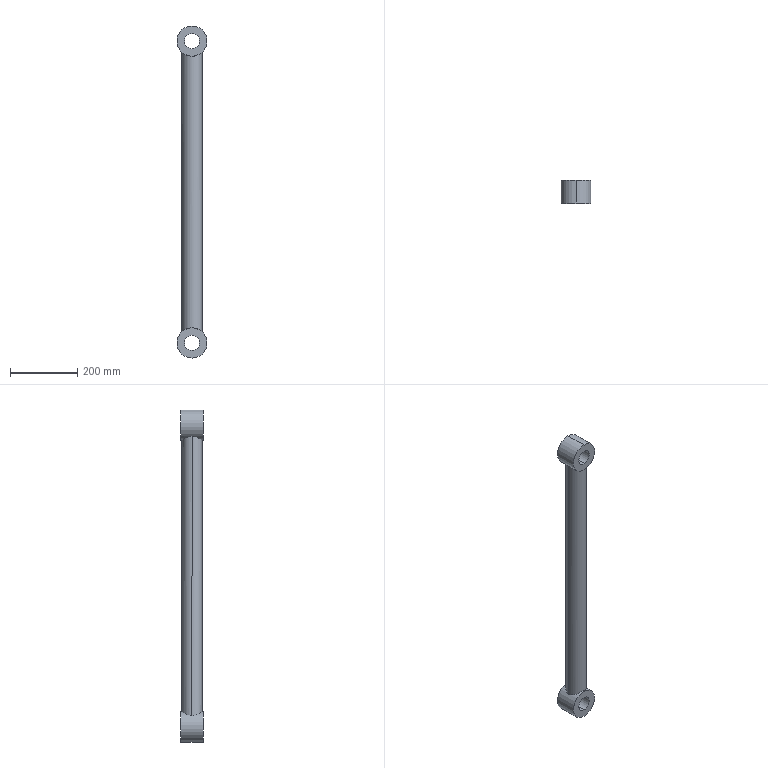Part | SolidWorks | features ICE 2, Extrusion 1, Scale 1 | 1 solid | 14 faces | box 90 x 67.5 x 990 mm | volume 2949409 mm3 | cylinder 10 | plane 4 | commonest cylinder face diameters 45 x4 90 x4 60 x2
STEP:
#1=CARTESIAN_POINT('',(0.00000416,33.75,-472.5));
#2=VERTEX_POINT('',#1);
#3=CARTESIAN_POINT('',(0.00000416,33.75,-427.5));
#4=VERTEX_POINT('',#3);
#5=CARTESIAN_POINT('',(0.00000416,33.75,-450.));
#6=DIRECTION('',(0.,1.,0.));
#7=DIRECTION('',(0.,0.,-1.));
#8=AXIS2_PLACEMENT_3D('',#5,#6,#7);
#9=CIRCLE('',#8,22.5);
#10=EDGE_CURVE('',#2,#4,#9,.T.);
#11=ORIENTED_EDGE('',*,*,#10,.T.);
#12=CARTESIAN_POINT('',(0.00000416,-33.75,-427.5));
#13=VERTEX_POINT('',#12);
#14=CARTESIAN_POINT('',(0.00000416,33.75,-427.5));
#15=DIRECTION('',(0.,-1.,0.));
#16=VECTOR('',#15,1000.);
#17=LINE('',#14,#16);
#18=EDGE_CURVE('',#4,#13,#17,.T.);
#19=ORIENTED_EDGE('',*,*,#18,.T.);
#20=CARTESIAN_POINT('',(0.00000416,-33.75,-472.5));
#21=VERTEX_POINT('',#20);
#22=CARTESIAN_POINT('',(0.00000416,-33.75,-450.));
#23=DIRECTION('',(0.,1.,0.));
#24=DIRECTION('',(0.,0.,-1.));
#25=AXIS2_PLACEMENT_3D('',#22,#23,#24);
#26=CIRCLE('',#25,22.5);
#27=EDGE_CURVE('',#21,#13,#26,.T.);
#28=ORIENTED_EDGE('',*,*,#27,.F.);
#29=CARTESIAN_POINT('',(0.00000416,33.75,-472.5));
#30=DIRECTION('',(0.,-1.,0.));
#31=VECTOR('',#30,1000.);
#32=LINE('',#29,#31);
#33=EDGE_CURVE('',#2,#21,#32,.T.);
#34=ORIENTED_EDGE('',*,*,#33,.F.);
#35=EDGE_LOOP('',(#11,#19,#28,#34));
#36=FACE_OUTER_BOUND('',#35,.T.);
#37=CARTESIAN_POINT('',(0.00000416,33.75,-450.));
#38=DIRECTION('',(0.,-1.,0.));
#39=DIRECTION('',(0.,0.,-1.));
#40=AXIS2_PLACEMENT_3D('',#37,#38,#39);
#41=CYLINDRICAL_SURFACE('',#40,22.5);
#42=ADVANCED_FACE('',(#36),#41,.F.);
#43=CARTESIAN_POINT('',(0.00000416,33.75,-405.));
#44=VERTEX_POINT('',#43);
#45=CARTESIAN_POINT('',(0.00000416,33.75,-495.));
#46=VERTEX_POINT('',#45);
#47=CARTESIAN_POINT('',(0.00000416,33.75,-450.));
#48=DIRECTION('',(0.,1.,0.));
#49=DIRECTION('',(0.,0.,-1.));
#50=AXIS2_PLACEMENT_3D('',#47,#48,#49);
#51=CIRCLE('',#50,45.);
#52=EDGE_CURVE('',#44,#46,#51,.T.);
#53=ORIENTED_EDGE('',*,*,#52,.F.);
#54=CARTESIAN_POINT('',(0.00000416,30.,-405.));
#55=VERTEX_POINT('',#54);
#56=CARTESIAN_POINT('',(0.00000416,33.75,-405.));
#57=DIRECTION('',(0.,-1.,0.));
#58=VECTOR('',#57,1000.);
#59=LINE('',#56,#58);
#60=EDGE_CURVE('',#44,#55,#59,.T.);
#61=ORIENTED_EDGE('',*,*,#60,.T.);
#62=CARTESIAN_POINT('',(30.,0.00002262,-416.459));
#63=VERTEX_POINT('',#62);
#64=CARTESIAN_POINT('',(0.00000416,30.,-405.));
#65=CARTESIAN_POINT('',(0.5109,30.,-405.));
#66=CARTESIAN_POINT('',(1.025,29.987,-405.009));
#67=CARTESIAN_POINT('',(2.044,29.935,-405.043));
#68=CARTESIAN_POINT('',(2.55,29.896,-405.069));
#69=CARTESIAN_POINT('',(4.059,29.741,-405.172));
#70=CARTESIAN_POINT('',(5.054,29.588,-405.274));
#71=CARTESIAN_POINT('',(7.02,29.184,-405.54));
#72=CARTESIAN_POINT('',(7.992,28.933,-405.704));
#73=CARTESIAN_POINT('',(9.913,28.333,-406.094));
#74=CARTESIAN_POINT('',(10.847,27.988,-406.317));
#75=CARTESIAN_POINT('',(12.659,27.216,-406.807));
#76=CARTESIAN_POINT('',(13.538,26.789,-407.075));
#77=CARTESIAN_POINT('',(14.82,26.089,-407.508));
#78=CARTESIAN_POINT('',(15.241,25.845,-407.657));
#79=CARTESIAN_POINT('',(16.07,25.338,-407.965));
#80=CARTESIAN_POINT('',(16.479,25.073,-408.124));
#81=CARTESIAN_POINT('',(18.483,23.709,-408.935));
#82=CARTESIAN_POINT('',(19.945,22.49,-409.633));
#83=CARTESIAN_POINT('',(21.951,20.471,-410.71));
#84=CARTESIAN_POINT('',(22.589,19.765,-411.074));
#85=CARTESIAN_POINT('',(23.801,18.288,-411.803));
#86=CARTESIAN_POINT('',(24.369,17.523,-412.164));
#87=CARTESIAN_POINT('',(25.958,15.158,-413.22));
#88=CARTESIAN_POINT('',(26.868,13.486,-413.888));
#89=CARTESIAN_POINT('',(27.814,11.252,-414.624));
#90=CARTESIAN_POINT('',(27.994,10.798,-414.766));
#91=CARTESIAN_POINT('',(28.333,9.875,-415.038));
#92=CARTESIAN_POINT('',(28.492,9.403,-415.169));
#93=CARTESIAN_POINT('',(28.936,7.981,-415.534));
#94=CARTESIAN_POINT('',(29.184,7.019,-415.746));
#95=CARTESIAN_POINT('',(29.587,5.063,-416.093));
#96=CARTESIAN_POINT('',(29.74,4.069,-416.228));
#97=CARTESIAN_POINT('',(29.895,2.553,-416.366));
#98=CARTESIAN_POINT('',(29.935,2.042,-416.401));
#99=CARTESIAN_POINT('',(29.987,1.019,-416.447));
#100=CARTESIAN_POINT('',(30.,0.5084,-416.459));
#101=CARTESIAN_POINT('',(30.,0.00002262,-416.459));
#102=B_SPLINE_CURVE_WITH_KNOTS('',3,(#64,#65,#66,#67,#68,#69,#70,#71,#72,#73,#74,#75,#76,#77,#78,#79,#80,#81,#82,#83,#84,#85,#86,#87,#88,#89,#90,#91,#92,#93,#94,#95,#96,#97,#98,#99,#100,#101),.UNSPECIFIED.,.F.,.F.,(4,2,2,2,2,2,2,2,2,2,2,2,2,2,2,2,2,2,4),(0.04853,0.05004,0.05155,0.05457,0.05759,0.06062,0.06364,0.06515,0.06666,0.07271,0.07573,0.07876,0.0848,0.08631,0.08783,0.09085,0.09387,0.09538,0.0969),.UNSPECIFIED.);
#103=EDGE_CURVE('',#55,#63,#102,.T.);
#104=ORIENTED_EDGE('',*,*,#103,.T.);
#105=CARTESIAN_POINT('',(0.00000416,-30.,-405.));
#106=VERTEX_POINT('',#105);
#107=CARTESIAN_POINT('',(30.,0.00002262,-416.459));
#108=CARTESIAN_POINT('',(30.,-2.032,-416.459));
#109=CARTESIAN_POINT('',(29.796,-4.037,-416.273));
#110=CARTESIAN_POINT('',(29.289,-6.511,-415.836));
#111=CARTESIAN_POINT('',(29.176,-7.001,-415.739));
#112=CARTESIAN_POINT('',(28.927,-7.968,-415.529));
#113=CARTESIAN_POINT('',(28.791,-8.445,-415.415));
#114=CARTESIAN_POINT('',(28.351,-9.859,-415.052));
#115=CARTESIAN_POINT('',(28.014,-10.778,-414.78));
#116=CARTESIAN_POINT('',(27.255,-12.574,-414.189));
#117=CARTESIAN_POINT('',(26.831,-13.455,-413.869));
#118=CARTESIAN_POINT('',(25.911,-15.15,-413.204));
#119=CARTESIAN_POINT('',(25.416,-15.967,-412.859));
#120=CARTESIAN_POINT('',(24.353,-17.546,-412.153));
#121=CARTESIAN_POINT('',(23.785,-18.307,-411.793));
#122=CARTESIAN_POINT('',(22.578,-19.778,-411.067));
#123=CARTESIAN_POINT('',(21.934,-20.489,-410.7));
#124=CARTESIAN_POINT('',(19.917,-22.516,-409.619));
#125=CARTESIAN_POINT('',(18.457,-23.728,-408.923));
#126=CARTESIAN_POINT('',(16.079,-25.345,-407.962));
#127=CARTESIAN_POINT('',(15.255,-25.851,-407.655));
#128=CARTESIAN_POINT('',(13.967,-26.555,-407.22));
#129=CARTESIAN_POINT('',(13.528,-26.781,-407.079));
#130=CARTESIAN_POINT('',(12.64,-27.212,-406.809));
#131=CARTESIAN_POINT('',(12.191,-27.416,-406.68));
#132=CARTESIAN_POINT('',(9.921,-28.381,-406.067));
#133=CARTESIAN_POINT('',(8.025,-28.977,-405.676));
#134=CARTESIAN_POINT('',(5.545,-29.487,-405.34));
#135=CARTESIAN_POINT('',(5.042,-29.578,-405.28));
#136=CARTESIAN_POINT('',(4.035,-29.732,-405.178));
#137=CARTESIAN_POINT('',(3.532,-29.796,-405.136));
#138=CARTESIAN_POINT('',(2.02,-29.949,-405.034));
#139=CARTESIAN_POINT('',(1.011,-30.,-405.));
#140=CARTESIAN_POINT('',(0.00000416,-30.,-405.));
#141=B_SPLINE_CURVE_WITH_KNOTS('',3,(#107,#108,#109,#110,#111,#112,#113,#114,#115,#116,#117,#118,#119,#120,#121,#122,#123,#124,#125,#126,#127,#128,#129,#130,#131,#132,#133,#134,#135,#136,#137,#138,#139,#140),.UNSPECIFIED.,.F.,.F.,(4,2,2,2,2,2,2,2,2,2,2,2,2,2,2,2,4),(0.0969,0.1029,0.1044,0.106,0.109,0.112,0.115,0.118,0.1211,0.1271,0.1301,0.1316,0.1331,0.1392,0.1407,0.1422,0.1452),.UNSPECIFIED.);
#142=EDGE_CURVE('',#63,#106,#141,.T.);
#143=ORIENTED_EDGE('',*,*,#142,.T.);
#144=CARTESIAN_POINT('',(0.00000416,-33.75,-405.));
#145=VERTEX_POINT('',#144);
#146=CARTESIAN_POINT('',(0.00000416,33.75,-405.));
#147=DIRECTION('',(0.,-1.,0.));
#148=VECTOR('',#147,1000.);
#149=LINE('',#146,#148);
#150=EDGE_CURVE('',#106,#145,#149,.T.);
#151=ORIENTED_EDGE('',*,*,#150,.T.);
#152=CARTESIAN_POINT('',(0.00000416,-33.75,-495.));
#153=VERTEX_POINT('',#152);
#154=CARTESIAN_POINT('',(0.00000416,-33.75,-450.));
#155=DIRECTION('',(0.,1.,0.));
#156=DIRECTION('',(0.,0.,-1.));
#157=AXIS2_PLACEMENT_3D('',#154,#155,#156);
#158=CIRCLE('',#157,45.);
#159=EDGE_CURVE('',#145,#153,#158,.T.);
#160=ORIENTED_EDGE('',*,*,#159,.T.);
#161=CARTESIAN_POINT('',(0.00000416,33.75,-495.));
#162=DIRECTION('',(0.,-1.,0.));
#163=VECTOR('',#162,1000.);
#164=LINE('',#161,#163);
#165=EDGE_CURVE('',#46,#153,#164,.T.);
#166=ORIENTED_EDGE('',*,*,#165,.F.);
#167=EDGE_LOOP('',(#53,#61,#104,#143,#151,#160,#166));
#168=FACE_OUTER_BOUND('',#167,.T.);
#169=CARTESIAN_POINT('',(0.00000416,33.75,-450.));
#170=DIRECTION('',(0.,-1.,0.));
#171=DIRECTION('',(0.,0.,-1.));
#172=AXIS2_PLACEMENT_3D('',#169,#170,#171);
#173=CYLINDRICAL_SURFACE('',#172,45.);
#174=ADVANCED_FACE('',(#168),#173,.T.);
#175=CARTESIAN_POINT('',(0.00000416,33.75,427.5));
#176=VERTEX_POINT('',#175);
#177=CARTESIAN_POINT('',(0.00000416,33.75,472.5));
#178=VERTEX_POINT('',#177);
#179=CARTESIAN_POINT('',(0.00000416,33.75,450.));
#180=DIRECTION('',(0.,1.,0.));
#181=DIRECTION('',(0.,0.,1.));
#182=AXIS2_PLACEMENT_3D('',#179,#180,#181);
#183=CIRCLE('',#182,22.5);
#184=EDGE_CURVE('',#176,#178,#183,.T.);
#185=ORIENTED_EDGE('',*,*,#184,.T.);
#186=CARTESIAN_POINT('',(0.00000416,-33.75,472.5));
#187=VERTEX_POINT('',#186);
#188=CARTESIAN_POINT('',(0.00000416,33.75,472.5));
#189=DIRECTION('',(0.,-1.,0.));
#190=VECTOR('',#189,1000.);
#191=LINE('',#188,#190);
#192=EDGE_CURVE('',#178,#187,#191,.T.);
#193=ORIENTED_EDGE('',*,*,#192,.T.);
#194=CARTESIAN_POINT('',(0.00000416,-33.75,427.5));
#195=VERTEX_POINT('',#194);
#196=CARTESIAN_POINT('',(0.00000416,-33.75,450.));
#197=DIRECTION('',(0.,1.,0.));
#198=DIRECTION('',(0.,0.,1.));
#199=AXIS2_PLACEMENT_3D('',#196,#197,#198);
#200=CIRCLE('',#199,22.5);
#201=EDGE_CURVE('',#195,#187,#200,.T.);
#202=ORIENTED_EDGE('',*,*,#201,.F.);
#203=CARTESIAN_POINT('',(0.00000416,33.75,427.5));
#204=DIRECTION('',(0.,-1.,0.));
#205=VECTOR('',#204,1000.);
#206=LINE('',#203,#205);
#207=EDGE_CURVE('',#176,#195,#206,.T.);
#208=ORIENTED_EDGE('',*,*,#207,.F.);
#209=EDGE_LOOP('',(#185,#193,#202,#208));
#210=FACE_OUTER_BOUND('',#209,.T.);
#211=CARTESIAN_POINT('',(0.00000416,33.75,450.));
#212=DIRECTION('',(0.,-1.,0.));
#213=DIRECTION('',(0.,0.,-1.));
#214=AXIS2_PLACEMENT_3D('',#211,#212,#213);
#215=CYLINDRICAL_SURFACE('',#214,22.5);
#216=ADVANCED_FACE('',(#210),#215,.F.);
#217=CARTESIAN_POINT('',(0.00000416,33.75,495.));
#218=VERTEX_POINT('',#217);
#219=CARTESIAN_POINT('',(0.00000416,33.75,405.));
#220=VERTEX_POINT('',#219);
#221=CARTESIAN_POINT('',(0.00000416,33.75,450.));
#222=DIRECTION('',(0.,1.,0.));
#223=DIRECTION('',(0.,0.,1.));
#224=AXIS2_PLACEMENT_3D('',#221,#222,#223);
#225=CIRCLE('',#224,45.);
#226=EDGE_CURVE('',#218,#220,#225,.T.);
#227=ORIENTED_EDGE('',*,*,#226,.F.);
#228=CARTESIAN_POINT('',(0.00000416,-33.75,495.));
#229=VERTEX_POINT('',#228);
#230=CARTESIAN_POINT('',(0.00000416,33.75,495.));
#231=DIRECTION('',(0.,-1.,0.));
#232=VECTOR('',#231,1000.);
#233=LINE('',#230,#232);
#234=EDGE_CURVE('',#218,#229,#233,.T.);
#235=ORIENTED_EDGE('',*,*,#234,.T.);
#236=CARTESIAN_POINT('',(0.00000416,-33.75,405.));
#237=VERTEX_POINT('',#236);
#238=CARTESIAN_POINT('',(0.00000416,-33.75,450.));
#239=DIRECTION('',(0.,1.,0.));
#240=DIRECTION('',(0.,0.,1.));
#241=AXIS2_PLACEMENT_3D('',#238,#239,#240);
#242=CIRCLE('',#241,45.);
#243=EDGE_CURVE('',#229,#237,#242,.T.);
#244=ORIENTED_EDGE('',*,*,#243,.T.);
#245=CARTESIAN_POINT('',(0.00000416,-30.,405.));
#246=VERTEX_POINT('',#245);
#247=CARTESIAN_POINT('',(0.00000416,33.75,405.));
#248=DIRECTION('',(0.,-1.,0.));
#249=VECTOR('',#248,1000.);
#250=LINE('',#247,#249);
#251=EDGE_CURVE('',#246,#237,#250,.T.);
#252=ORIENTED_EDGE('',*,*,#251,.F.);
#253=CARTESIAN_POINT('',(30.,0.00002262,416.459));
#254=VERTEX_POINT('',#253);
#255=CARTESIAN_POINT('',(0.00000416,-30.,405.));
#256=CARTESIAN_POINT('',(0.5109,-30.,405.));
#257=CARTESIAN_POINT('',(1.025,-29.987,405.009));
#258=CARTESIAN_POINT('',(2.044,-29.935,405.044));
#259=CARTESIAN_POINT('',(2.55,-29.896,405.07));
#260=CARTESIAN_POINT('',(4.059,-29.741,405.172));
#261=CARTESIAN_POINT('',(5.054,-29.588,405.274));
#262=CARTESIAN_POINT('',(7.02,-29.184,405.54));
#263=CARTESIAN_POINT('',(7.992,-28.933,405.705));
#264=CARTESIAN_POINT('',(9.913,-28.333,406.095));
#265=CARTESIAN_POINT('',(10.847,-27.988,406.317));
#266=CARTESIAN_POINT('',(12.659,-27.216,406.807));
#267=CARTESIAN_POINT('',(13.538,-26.789,407.075));
#268=CARTESIAN_POINT('',(14.82,-26.089,407.508));
#269=CARTESIAN_POINT('',(15.241,-25.845,407.657));
#270=CARTESIAN_POINT('',(16.07,-25.338,407.965));
#271=CARTESIAN_POINT('',(16.479,-25.073,408.124));
#272=CARTESIAN_POINT('',(18.483,-23.709,408.935));
#273=CARTESIAN_POINT('',(19.945,-22.49,409.633));
#274=CARTESIAN_POINT('',(21.951,-20.47,410.71));
#275=CARTESIAN_POINT('',(22.589,-19.765,411.074));
#276=CARTESIAN_POINT('',(23.801,-18.288,411.803));
#277=CARTESIAN_POINT('',(24.369,-17.523,412.164));
#278=CARTESIAN_POINT('',(25.958,-15.158,413.22));
#279=CARTESIAN_POINT('',(26.868,-13.486,413.889));
#280=CARTESIAN_POINT('',(27.814,-11.252,414.624));
#281=CARTESIAN_POINT('',(27.994,-10.798,414.766));
#282=CARTESIAN_POINT('',(28.333,-9.875,415.039));
#283=CARTESIAN_POINT('',(28.492,-9.403,415.169));
#284=CARTESIAN_POINT('',(28.936,-7.981,415.535));
#285=CARTESIAN_POINT('',(29.184,-7.019,415.746));
#286=CARTESIAN_POINT('',(29.587,-5.063,416.093));
#287=CARTESIAN_POINT('',(29.74,-4.069,416.228));
#288=CARTESIAN_POINT('',(29.895,-2.553,416.366));
#289=CARTESIAN_POINT('',(29.935,-2.042,416.401));
#290=CARTESIAN_POINT('',(29.987,-1.019,416.448));
#291=CARTESIAN_POINT('',(30.,-0.5084,416.459));
#292=CARTESIAN_POINT('',(30.,0.00002262,416.459));
#293=B_SPLINE_CURVE_WITH_KNOTS('',3,(#255,#256,#257,#258,#259,#260,#261,#262,#263,#264,#265,#266,#267,#268,#269,#270,#271,#272,#273,#274,#275,#276,#277,#278,#279,#280,#281,#282,#283,#284,#285,#286,#287,#288,#289,#290,#291,#292),.UNSPECIFIED.,.F.,.F.,(4,2,2,2,2,2,2,2,2,2,2,2,2,2,2,2,2,2,4),(0.04853,0.05004,0.05155,0.05457,0.05759,0.06062,0.06364,0.06515,0.06666,0.07271,0.07573,0.07876,0.0848,0.08631,0.08783,0.09085,0.09387,0.09538,0.0969),.UNSPECIFIED.);
#294=EDGE_CURVE('',#246,#254,#293,.T.);
#295=ORIENTED_EDGE('',*,*,#294,.T.);
#296=CARTESIAN_POINT('',(0.00000416,30.,405.));
#297=VERTEX_POINT('',#296);
#298=CARTESIAN_POINT('',(30.,0.00002262,416.459));
#299=CARTESIAN_POINT('',(30.,2.032,416.459));
#300=CARTESIAN_POINT('',(29.796,4.037,416.273));
#301=CARTESIAN_POINT('',(29.289,6.511,415.836));
#302=CARTESIAN_POINT('',(29.176,7.002,415.739));
#303=CARTESIAN_POINT('',(28.927,7.968,415.529));
#304=CARTESIAN_POINT('',(28.791,8.445,415.415));
#305=CARTESIAN_POINT('',(28.351,9.859,415.052));
#306=CARTESIAN_POINT('',(28.014,10.778,414.78));
#307=CARTESIAN_POINT('',(27.255,12.574,414.19));
#308=CARTESIAN_POINT('',(26.831,13.455,413.87));
#309=CARTESIAN_POINT('',(25.911,15.15,413.205));
#310=CARTESIAN_POINT('',(25.416,15.967,412.859));
#311=CARTESIAN_POINT('',(24.353,17.546,412.154));
#312=CARTESIAN_POINT('',(23.785,18.307,411.793));
#313=CARTESIAN_POINT('',(22.578,19.778,411.068));
#314=CARTESIAN_POINT('',(21.934,20.489,410.7));
#315=CARTESIAN_POINT('',(19.917,22.516,409.619));
#316=CARTESIAN_POINT('',(18.457,23.728,408.924));
#317=CARTESIAN_POINT('',(16.079,25.346,407.962));
#318=CARTESIAN_POINT('',(15.255,25.851,407.655));
#319=CARTESIAN_POINT('',(13.967,26.555,407.22));
#320=CARTESIAN_POINT('',(13.528,26.781,407.079));
#321=CARTESIAN_POINT('',(12.64,27.212,406.809));
#322=CARTESIAN_POINT('',(12.191,27.416,406.68));
#323=CARTESIAN_POINT('',(9.921,28.381,406.067));
#324=CARTESIAN_POINT('',(8.025,28.978,405.676));
#325=CARTESIAN_POINT('',(5.545,29.487,405.34));
#326=CARTESIAN_POINT('',(5.042,29.578,405.281));
#327=CARTESIAN_POINT('',(4.035,29.732,405.179));
#328=CARTESIAN_POINT('',(3.532,29.796,405.136));
#329=CARTESIAN_POINT('',(2.02,29.949,405.034));
#330=CARTESIAN_POINT('',(1.011,30.,405.));
#331=CARTESIAN_POINT('',(0.00000416,30.,405.));
#332=B_SPLINE_CURVE_WITH_KNOTS('',3,(#298,#299,#300,#301,#302,#303,#304,#305,#306,#307,#308,#309,#310,#311,#312,#313,#314,#315,#316,#317,#318,#319,#320,#321,#322,#323,#324,#325,#326,#327,#328,#329,#330,#331),.UNSPECIFIED.,.F.,.F.,(4,2,2,2,2,2,2,2,2,2,2,2,2,2,2,2,4),(0.0969,0.1029,0.1044,0.106,0.109,0.112,0.115,0.118,0.1211,0.1271,0.1301,0.1316,0.1331,0.1392,0.1407,0.1422,0.1452),.UNSPECIFIED.);
#333=EDGE_CURVE('',#254,#297,#332,.T.);
#334=ORIENTED_EDGE('',*,*,#333,.T.);
#335=CARTESIAN_POINT('',(0.00000416,33.75,405.));
#336=DIRECTION('',(0.,-1.,0.));
#337=VECTOR('',#336,1000.);
#338=LINE('',#335,#337);
#339=EDGE_CURVE('',#220,#297,#338,.T.);
#340=ORIENTED_EDGE('',*,*,#339,.F.);
#341=EDGE_LOOP('',(#227,#235,#244,#252,#295,#334,#340));
#342=FACE_OUTER_BOUND('',#341,.T.);
#343=CARTESIAN_POINT('',(0.00000416,33.75,450.));
#344=DIRECTION('',(0.,-1.,0.));
#345=DIRECTION('',(0.,0.,-1.));
#346=AXIS2_PLACEMENT_3D('',#343,#344,#345);
#347=CYLINDRICAL_SURFACE('',#346,45.);
#348=ADVANCED_FACE('',(#342),#347,.T.);
#349=ORIENTED_EDGE('',*,*,#333,.F.);
#350=CARTESIAN_POINT('',(30.,0.00002262,450.));
#351=DIRECTION('',(0.,0.,-1.));
#352=VECTOR('',#351,1000.);
#353=LINE('',#350,#352);
#354=EDGE_CURVE('',#254,#63,#353,.T.);
#355=ORIENTED_EDGE('',*,*,#354,.T.);
#356=ORIENTED_EDGE('',*,*,#103,.F.);
#357=CARTESIAN_POINT('',(-30.,0.00002262,-416.459));
#358=VERTEX_POINT('',#357);
#359=CARTESIAN_POINT('',(-30.,0.00002262,-416.459));
#360=CARTESIAN_POINT('',(-30.,2.059,-416.459));
#361=CARTESIAN_POINT('',(-29.791,4.064,-416.269));
#362=CARTESIAN_POINT('',(-29.289,6.51,-415.836));
#363=CARTESIAN_POINT('',(-29.177,6.996,-415.74));
#364=CARTESIAN_POINT('',(-28.928,7.963,-415.53));
#365=CARTESIAN_POINT('',(-28.791,8.445,-415.415));
#366=CARTESIAN_POINT('',(-28.347,9.871,-415.048));
#367=CARTESIAN_POINT('',(-28.008,10.793,-414.775));
#368=CARTESIAN_POINT('',(-27.25,12.584,-414.186));
#369=CARTESIAN_POINT('',(-26.831,13.454,-413.869));
#370=CARTESIAN_POINT('',(-26.143,14.724,-413.372));
#371=CARTESIAN_POINT('',(-25.903,15.141,-413.202));
#372=CARTESIAN_POINT('',(-25.404,15.964,-412.855));
#373=CARTESIAN_POINT('',(-25.144,16.371,-412.679));
#374=CARTESIAN_POINT('',(-23.805,18.358,-411.79));
#375=CARTESIAN_POINT('',(-22.601,19.82,-411.057));
#376=CARTESIAN_POINT('',(-20.589,21.84,-409.979));
#377=CARTESIAN_POINT('',(-19.884,22.485,-409.623));
#378=CARTESIAN_POINT('',(-18.399,23.715,-408.925));
#379=CARTESIAN_POINT('',(-17.629,24.293,-408.588));
#380=CARTESIAN_POINT('',(-15.244,25.91,-407.626));
#381=CARTESIAN_POINT('',(-13.55,26.838,-407.047));
#382=CARTESIAN_POINT('',(-11.285,27.801,-406.435));
#383=CARTESIAN_POINT('',(-10.825,27.983,-406.319));
#384=CARTESIAN_POINT('',(-9.889,28.328,-406.097));
#385=CARTESIAN_POINT('',(-9.411,28.49,-405.992));
#386=CARTESIAN_POINT('',(-7.971,28.939,-405.701));
#387=CARTESIAN_POINT('',(-7.,29.189,-405.537));
#388=CARTESIAN_POINT('',(-4.055,29.792,-405.139));
#389=CARTESIAN_POINT('',(-2.05,30.,-405.));
#390=CARTESIAN_POINT('',(0.00000416,30.,-405.));
#391=B_SPLINE_CURVE_WITH_KNOTS('',3,(#359,#360,#361,#362,#363,#364,#365,#366,#367,#368,#369,#370,#371,#372,#373,#374,#375,#376,#377,#378,#379,#380,#381,#382,#383,#384,#385,#386,#387,#388,#389,#390),.UNSPECIFIED.,.F.,.F.,(4,2,2,2,2,2,2,2,2,2,2,2,2,2,2,4),(0.,0.006066,0.007582,0.009099,0.01213,0.01516,0.01668,0.0182,0.02426,0.0273,0.03033,0.03639,0.03791,0.03943,0.04246,0.04853),.UNSPECIFIED.);
#392=EDGE_CURVE('',#358,#55,#391,.T.);
#393=ORIENTED_EDGE('',*,*,#392,.F.);
#394=CARTESIAN_POINT('',(-30.,0.00002262,416.459));
#395=VERTEX_POINT('',#394);
#396=CARTESIAN_POINT('',(-30.,0.00002262,450.));
#397=DIRECTION('',(0.,0.,-1.));
#398=VECTOR('',#397,1000.);
#399=LINE('',#396,#398);
#400=EDGE_CURVE('',#395,#358,#399,.T.);
#401=ORIENTED_EDGE('',*,*,#400,.F.);
#402=CARTESIAN_POINT('',(0.00000416,30.,405.));
#403=CARTESIAN_POINT('',(-1.009,30.,405.));
#404=CARTESIAN_POINT('',(-2.02,29.949,405.034));
#405=CARTESIAN_POINT('',(-3.539,29.795,405.137));
#406=CARTESIAN_POINT('',(-4.047,29.73,405.18));
#407=CARTESIAN_POINT('',(-5.052,29.576,405.282));
#408=CARTESIAN_POINT('',(-5.55,29.486,405.341));
#409=CARTESIAN_POINT('',(-8.016,28.979,405.675));
#410=CARTESIAN_POINT('',(-9.914,28.384,406.065));
#411=CARTESIAN_POINT('',(-12.656,27.218,406.806));
#412=CARTESIAN_POINT('',(-13.542,26.787,407.077));
#413=CARTESIAN_POINT('',(-15.25,25.853,407.653));
#414=CARTESIAN_POINT('',(-16.073,25.349,407.96));
#415=CARTESIAN_POINT('',(-17.665,24.267,408.603));
#416=CARTESIAN_POINT('',(-18.433,23.689,408.94));
#417=CARTESIAN_POINT('',(-19.913,22.459,409.638));
#418=CARTESIAN_POINT('',(-20.617,21.814,409.993));
#419=CARTESIAN_POINT('',(-22.622,19.795,411.07));
#420=CARTESIAN_POINT('',(-23.821,18.337,411.8));
#421=CARTESIAN_POINT('',(-25.421,15.96,412.862));
#422=CARTESIAN_POINT('',(-25.921,15.133,413.211));
#423=CARTESIAN_POINT('',(-26.837,13.443,413.874));
#424=CARTESIAN_POINT('',(-27.254,12.576,414.189));
#425=CARTESIAN_POINT('',(-28.008,10.793,414.776));
#426=CARTESIAN_POINT('',(-28.345,9.877,415.047));
#427=CARTESIAN_POINT('',(-28.933,7.991,415.532));
#428=CARTESIAN_POINT('',(-29.186,7.015,415.747));
#429=CARTESIAN_POINT('',(-29.589,5.048,416.095));
#430=CARTESIAN_POINT('',(-29.742,4.053,416.23));
#431=CARTESIAN_POINT('',(-29.896,2.546,416.366));
#432=CARTESIAN_POINT('',(-29.935,2.041,416.401));
#433=CARTESIAN_POINT('',(-29.987,1.025,416.447));
#434=CARTESIAN_POINT('',(-30.,0.5121,416.459));
#435=CARTESIAN_POINT('',(-30.,0.00002262,416.459));
#436=B_SPLINE_CURVE_WITH_KNOTS('',3,(#402,#403,#404,#405,#406,#407,#408,#409,#410,#411,#412,#413,#414,#415,#416,#417,#418,#419,#420,#421,#422,#423,#424,#425,#426,#427,#428,#429,#430,#431,#432,#433,#434,#435),.UNSPECIFIED.,.F.,.F.,(4,2,2,2,2,2,2,2,2,2,2,2,2,2,2,2,4),(0.1452,0.1482,0.1498,0.1513,0.1573,0.1603,0.1633,0.1664,0.1694,0.1754,0.1784,0.1814,0.1845,0.1875,0.1905,0.192,0.1935),.UNSPECIFIED.);
#437=EDGE_CURVE('',#297,#395,#436,.T.);
#438=ORIENTED_EDGE('',*,*,#437,.F.);
#439=EDGE_LOOP('',(#349,#355,#356,#393,#401,#438));
#440=FACE_OUTER_BOUND('',#439,.T.);
#441=CARTESIAN_POINT('',(0.00000416,0.00002262,450.));
#442=DIRECTION('',(0.,0.,-1.));
#443=DIRECTION('',(-1.,0.,0.));
#444=AXIS2_PLACEMENT_3D('',#441,#442,#443);
#445=CYLINDRICAL_SURFACE('',#444,30.);
#446=ADVANCED_FACE('',(#440),#445,.T.);
#447=ORIENTED_EDGE('',*,*,#354,.F.);
#448=ORIENTED_EDGE('',*,*,#294,.F.);
#449=CARTESIAN_POINT('',(-30.,0.00002262,416.459));
#450=CARTESIAN_POINT('',(-30.,-2.059,416.459));
#451=CARTESIAN_POINT('',(-29.791,-4.064,416.269));
#452=CARTESIAN_POINT('',(-29.289,-6.51,415.837));
#453=CARTESIAN_POINT('',(-29.177,-6.996,415.74));
#454=CARTESIAN_POINT('',(-28.928,-7.963,415.53));
#455=CARTESIAN_POINT('',(-28.791,-8.445,415.415));
#456=CARTESIAN_POINT('',(-28.347,-9.871,415.049));
#457=CARTESIAN_POINT('',(-28.008,-10.793,414.776));
#458=CARTESIAN_POINT('',(-27.25,-12.584,414.186));
#459=CARTESIAN_POINT('',(-26.831,-13.454,413.87));
#460=CARTESIAN_POINT('',(-26.143,-14.724,413.372));
#461=CARTESIAN_POINT('',(-25.903,-15.141,413.202));
#462=CARTESIAN_POINT('',(-25.404,-15.964,412.856));
#463=CARTESIAN_POINT('',(-25.144,-16.37,412.679));
#464=CARTESIAN_POINT('',(-23.805,-18.358,411.79));
#465=CARTESIAN_POINT('',(-22.601,-19.819,411.058));
#466=CARTESIAN_POINT('',(-20.589,-21.84,409.979));
#467=CARTESIAN_POINT('',(-19.884,-22.485,409.623));
#468=CARTESIAN_POINT('',(-18.399,-23.715,408.925));
#469=CARTESIAN_POINT('',(-17.629,-24.293,408.588));
#470=CARTESIAN_POINT('',(-15.244,-25.91,407.626));
#471=CARTESIAN_POINT('',(-13.55,-26.838,407.047));
#472=CARTESIAN_POINT('',(-11.285,-27.801,406.436));
#473=CARTESIAN_POINT('',(-10.825,-27.983,406.319));
#474=CARTESIAN_POINT('',(-9.889,-28.328,406.097));
#475=CARTESIAN_POINT('',(-9.411,-28.49,405.993));
#476=CARTESIAN_POINT('',(-7.971,-28.939,405.701));
#477=CARTESIAN_POINT('',(-7.,-29.189,405.537));
#478=CARTESIAN_POINT('',(-4.055,-29.792,405.139));
#479=CARTESIAN_POINT('',(-2.05,-30.,405.));
#480=CARTESIAN_POINT('',(0.00000416,-30.,405.));
#481=B_SPLINE_CURVE_WITH_KNOTS('',3,(#449,#450,#451,#452,#453,#454,#455,#456,#457,#458,#459,#460,#461,#462,#463,#464,#465,#466,#467,#468,#469,#470,#471,#472,#473,#474,#475,#476,#477,#478,#479,#480),.UNSPECIFIED.,.F.,.F.,(4,2,2,2,2,2,2,2,2,2,2,2,2,2,2,4),(0.,0.006066,0.007582,0.009099,0.01213,0.01516,0.01668,0.0182,0.02426,0.0273,0.03033,0.03639,0.03791,0.03943,0.04246,0.04853),.UNSPECIFIED.);
#482=EDGE_CURVE('',#395,#246,#481,.T.);
#483=ORIENTED_EDGE('',*,*,#482,.F.);
#484=ORIENTED_EDGE('',*,*,#400,.T.);
#485=CARTESIAN_POINT('',(0.00000416,-30.,-405.));
#486=CARTESIAN_POINT('',(-1.009,-30.,-405.));
#487=CARTESIAN_POINT('',(-2.02,-29.949,-405.034));
#488=CARTESIAN_POINT('',(-3.539,-29.795,-405.136));
#489=CARTESIAN_POINT('',(-4.047,-29.73,-405.179));
#490=CARTESIAN_POINT('',(-5.052,-29.576,-405.282));
#491=CARTESIAN_POINT('',(-5.55,-29.486,-405.341));
#492=CARTESIAN_POINT('',(-8.016,-28.979,-405.675));
#493=CARTESIAN_POINT('',(-9.914,-28.384,-406.065));
#494=CARTESIAN_POINT('',(-12.656,-27.218,-406.806));
#495=CARTESIAN_POINT('',(-13.542,-26.787,-407.076));
#496=CARTESIAN_POINT('',(-15.25,-25.853,-407.653));
#497=CARTESIAN_POINT('',(-16.073,-25.349,-407.96));
#498=CARTESIAN_POINT('',(-17.665,-24.267,-408.603));
#499=CARTESIAN_POINT('',(-18.433,-23.689,-408.94));
#500=CARTESIAN_POINT('',(-19.913,-22.459,-409.637));
#501=CARTESIAN_POINT('',(-20.617,-21.814,-409.993));
#502=CARTESIAN_POINT('',(-22.622,-19.795,-411.07));
#503=CARTESIAN_POINT('',(-23.821,-18.337,-411.8));
#504=CARTESIAN_POINT('',(-25.421,-15.96,-412.862));
#505=CARTESIAN_POINT('',(-25.921,-15.133,-413.211));
#506=CARTESIAN_POINT('',(-26.837,-13.443,-413.874));
#507=CARTESIAN_POINT('',(-27.254,-12.576,-414.189));
#508=CARTESIAN_POINT('',(-28.008,-10.793,-414.775));
#509=CARTESIAN_POINT('',(-28.345,-9.877,-415.047));
#510=CARTESIAN_POINT('',(-28.933,-7.991,-415.532));
#511=CARTESIAN_POINT('',(-29.186,-7.015,-415.747));
#512=CARTESIAN_POINT('',(-29.589,-5.047,-416.095));
#513=CARTESIAN_POINT('',(-29.742,-4.053,-416.23));
#514=CARTESIAN_POINT('',(-29.896,-2.546,-416.366));
#515=CARTESIAN_POINT('',(-29.935,-2.041,-416.401));
#516=CARTESIAN_POINT('',(-29.987,-1.025,-416.447));
#517=CARTESIAN_POINT('',(-30.,-0.512,-416.459));
#518=CARTESIAN_POINT('',(-30.,0.00002262,-416.459));
#519=B_SPLINE_CURVE_WITH_KNOTS('',3,(#485,#486,#487,#488,#489,#490,#491,#492,#493,#494,#495,#496,#497,#498,#499,#500,#501,#502,#503,#504,#505,#506,#507,#508,#509,#510,#511,#512,#513,#514,#515,#516,#517,#518),.UNSPECIFIED.,.F.,.F.,(4,2,2,2,2,2,2,2,2,2,2,2,2,2,2,2,4),(0.1452,0.1482,0.1498,0.1513,0.1573,0.1603,0.1633,0.1664,0.1694,0.1754,0.1784,0.1814,0.1845,0.1875,0.1905,0.192,0.1935),.UNSPECIFIED.);
#520=EDGE_CURVE('',#106,#358,#519,.T.);
#521=ORIENTED_EDGE('',*,*,#520,.F.);
#522=ORIENTED_EDGE('',*,*,#142,.F.);
#523=EDGE_LOOP('',(#447,#448,#483,#484,#521,#522));
#524=FACE_OUTER_BOUND('',#523,.T.);
#525=CARTESIAN_POINT('',(0.00000416,0.00002262,450.));
#526=DIRECTION('',(0.,0.,-1.));
#527=DIRECTION('',(-1.,0.,0.));
#528=AXIS2_PLACEMENT_3D('',#525,#526,#527);
#529=CYLINDRICAL_SURFACE('',#528,30.);
#530=ADVANCED_FACE('',(#524),#529,.T.);
#531=ORIENTED_EDGE('',*,*,#234,.F.);
#532=CARTESIAN_POINT('',(0.00000416,33.75,450.));
#533=DIRECTION('',(0.,1.,0.));
#534=DIRECTION('',(0.,0.,1.));
#535=AXIS2_PLACEMENT_3D('',#532,#533,#534);
#536=CIRCLE('',#535,45.);
#537=EDGE_CURVE('',#220,#218,#536,.T.);
#538=ORIENTED_EDGE('',*,*,#537,.F.);
#539=ORIENTED_EDGE('',*,*,#339,.T.);
#540=ORIENTED_EDGE('',*,*,#437,.T.);
#541=ORIENTED_EDGE('',*,*,#482,.T.);
#542=ORIENTED_EDGE('',*,*,#251,.T.);
#543=CARTESIAN_POINT('',(0.00000416,-33.75,450.));
#544=DIRECTION('',(0.,1.,0.));
#545=DIRECTION('',(0.,0.,1.));
#546=AXIS2_PLACEMENT_3D('',#543,#544,#545);
#547=CIRCLE('',#546,45.);
#548=EDGE_CURVE('',#237,#229,#547,.T.);
#549=ORIENTED_EDGE('',*,*,#548,.T.);
#550=EDGE_LOOP('',(#531,#538,#539,#540,#541,#542,#549));
#551=FACE_OUTER_BOUND('',#550,.T.);
#552=CARTESIAN_POINT('',(0.00000416,33.75,450.));
#553=DIRECTION('',(0.,-1.,0.));
#554=DIRECTION('',(0.,0.,-1.));
#555=AXIS2_PLACEMENT_3D('',#552,#553,#554);
#556=CYLINDRICAL_SURFACE('',#555,45.);
#557=ADVANCED_FACE('',(#551),#556,.T.);
#558=ORIENTED_EDGE('',*,*,#537,.T.);
#559=ORIENTED_EDGE('',*,*,#226,.T.);
#560=EDGE_LOOP('',(#558,#559));
#561=FACE_OUTER_BOUND('',#560,.T.);
#562=ORIENTED_EDGE('',*,*,#184,.F.);
#563=CARTESIAN_POINT('',(0.00000416,33.75,450.));
#564=DIRECTION('',(0.,1.,0.));
#565=DIRECTION('',(0.,0.,1.));
#566=AXIS2_PLACEMENT_3D('',#563,#564,#565);
#567=CIRCLE('',#566,22.5);
#568=EDGE_CURVE('',#178,#176,#567,.T.);
#569=ORIENTED_EDGE('',*,*,#568,.F.);
#570=EDGE_LOOP('',(#562,#569));
#571=FACE_BOUND('',#570,.T.);
#572=CARTESIAN_POINT('',(0.00000416,33.75,450.));
#573=DIRECTION('',(0.,1.,0.));
#574=DIRECTION('',(0.,0.,1.));
#575=AXIS2_PLACEMENT_3D('',#572,#573,#574);
#576=PLANE('',#575);
#577=ADVANCED_FACE('',(#561,#571),#576,.T.);
#578=ORIENTED_EDGE('',*,*,#548,.F.);
#579=ORIENTED_EDGE('',*,*,#243,.F.);
#580=EDGE_LOOP('',(#578,#579));
#581=FACE_OUTER_BOUND('',#580,.T.);
#582=ORIENTED_EDGE('',*,*,#201,.T.);
#583=CARTESIAN_POINT('',(0.00000416,-33.75,450.));
#584=DIRECTION('',(0.,1.,0.));
#585=DIRECTION('',(0.,0.,1.));
#586=AXIS2_PLACEMENT_3D('',#583,#584,#585);
#587=CIRCLE('',#586,22.5);
#588=EDGE_CURVE('',#187,#195,#587,.T.);
#589=ORIENTED_EDGE('',*,*,#588,.T.);
#590=EDGE_LOOP('',(#582,#589));
#591=FACE_BOUND('',#590,.T.);
#592=CARTESIAN_POINT('',(0.00000416,-33.75,450.));
#593=DIRECTION('',(0.,1.,0.));
#594=DIRECTION('',(0.,0.,1.));
#595=AXIS2_PLACEMENT_3D('',#592,#593,#594);
#596=PLANE('',#595);
#597=ADVANCED_FACE('',(#581,#591),#596,.F.);
#598=ORIENTED_EDGE('',*,*,#192,.F.);
#599=ORIENTED_EDGE('',*,*,#568,.T.);
#600=ORIENTED_EDGE('',*,*,#207,.T.);
#601=ORIENTED_EDGE('',*,*,#588,.F.);
#602=EDGE_LOOP('',(#598,#599,#600,#601));
#603=FACE_OUTER_BOUND('',#602,.T.);
#604=CARTESIAN_POINT('',(0.00000416,33.75,450.));
#605=DIRECTION('',(0.,-1.,0.));
#606=DIRECTION('',(0.,0.,-1.));
#607=AXIS2_PLACEMENT_3D('',#604,#605,#606);
#608=CYLINDRICAL_SURFACE('',#607,22.5);
#609=ADVANCED_FACE('',(#603),#608,.F.);
#610=ORIENTED_EDGE('',*,*,#60,.F.);
#611=CARTESIAN_POINT('',(0.00000416,33.75,-450.));
#612=DIRECTION('',(0.,1.,0.));
#613=DIRECTION('',(0.,0.,-1.));
#614=AXIS2_PLACEMENT_3D('',#611,#612,#613);
#615=CIRCLE('',#614,45.);
#616=EDGE_CURVE('',#46,#44,#615,.T.);
#617=ORIENTED_EDGE('',*,*,#616,.F.);
#618=ORIENTED_EDGE('',*,*,#165,.T.);
#619=CARTESIAN_POINT('',(0.00000416,-33.75,-450.));
#620=DIRECTION('',(0.,1.,0.));
#621=DIRECTION('',(0.,0.,-1.));
#622=AXIS2_PLACEMENT_3D('',#619,#620,#621);
#623=CIRCLE('',#622,45.);
#624=EDGE_CURVE('',#153,#145,#623,.T.);
#625=ORIENTED_EDGE('',*,*,#624,.T.);
#626=ORIENTED_EDGE('',*,*,#150,.F.);
#627=ORIENTED_EDGE('',*,*,#520,.T.);
#628=ORIENTED_EDGE('',*,*,#392,.T.);
#629=EDGE_LOOP('',(#610,#617,#618,#625,#626,#627,#628));
#630=FACE_OUTER_BOUND('',#629,.T.);
#631=CARTESIAN_POINT('',(0.00000416,33.75,-450.));
#632=DIRECTION('',(0.,-1.,0.));
#633=DIRECTION('',(0.,0.,-1.));
#634=AXIS2_PLACEMENT_3D('',#631,#632,#633);
#635=CYLINDRICAL_SURFACE('',#634,45.);
#636=ADVANCED_FACE('',(#630),#635,.T.);
#637=ORIENTED_EDGE('',*,*,#18,.F.);
#638=CARTESIAN_POINT('',(0.00000416,33.75,-450.));
#639=DIRECTION('',(0.,1.,0.));
#640=DIRECTION('',(0.,0.,-1.));
#641=AXIS2_PLACEMENT_3D('',#638,#639,#640);
#642=CIRCLE('',#641,22.5);
#643=EDGE_CURVE('',#4,#2,#642,.T.);
#644=ORIENTED_EDGE('',*,*,#643,.T.);
#645=ORIENTED_EDGE('',*,*,#33,.T.);
#646=CARTESIAN_POINT('',(0.00000416,-33.75,-450.));
#647=DIRECTION('',(0.,1.,0.));
#648=DIRECTION('',(0.,0.,-1.));
#649=AXIS2_PLACEMENT_3D('',#646,#647,#648);
#650=CIRCLE('',#649,22.5);
#651=EDGE_CURVE('',#13,#21,#650,.T.);
#652=ORIENTED_EDGE('',*,*,#651,.F.);
#653=EDGE_LOOP('',(#637,#644,#645,#652));
#654=FACE_OUTER_BOUND('',#653,.T.);
#655=CARTESIAN_POINT('',(0.00000416,33.75,-450.));
#656=DIRECTION('',(0.,-1.,0.));
#657=DIRECTION('',(0.,0.,-1.));
#658=AXIS2_PLACEMENT_3D('',#655,#656,#657);
#659=CYLINDRICAL_SURFACE('',#658,22.5);
#660=ADVANCED_FACE('',(#654),#659,.F.);
#661=ORIENTED_EDGE('',*,*,#616,.T.);
#662=ORIENTED_EDGE('',*,*,#52,.T.);
#663=EDGE_LOOP('',(#661,#662));
#664=FACE_OUTER_BOUND('',#663,.T.);
#665=ORIENTED_EDGE('',*,*,#10,.F.);
#666=ORIENTED_EDGE('',*,*,#643,.F.);
#667=EDGE_LOOP('',(#665,#666));
#668=FACE_BOUND('',#667,.T.);
#669=CARTESIAN_POINT('',(0.00000416,33.75,-450.));
#670=DIRECTION('',(0.,-1.,0.));
#671=DIRECTION('',(0.,0.,-1.));
#672=AXIS2_PLACEMENT_3D('',#669,#670,#671);
#673=PLANE('',#672);
#674=ADVANCED_FACE('',(#664,#668),#673,.F.);
#675=ORIENTED_EDGE('',*,*,#624,.F.);
#676=ORIENTED_EDGE('',*,*,#159,.F.);
#677=EDGE_LOOP('',(#675,#676));
#678=FACE_OUTER_BOUND('',#677,.T.);
#679=ORIENTED_EDGE('',*,*,#27,.T.);
#680=ORIENTED_EDGE('',*,*,#651,.T.);
#681=EDGE_LOOP('',(#679,#680));
#682=FACE_BOUND('',#681,.T.);
#683=CARTESIAN_POINT('',(0.00000416,-33.75,-450.));
#684=DIRECTION('',(0.,-1.,0.));
#685=DIRECTION('',(0.,0.,-1.));
#686=AXIS2_PLACEMENT_3D('',#683,#684,#685);
#687=PLANE('',#686);
#688=ADVANCED_FACE('',(#678,#682),#687,.T.);
#689=CLOSED_SHELL('',(#42,#174,#216,#348,#446,#530,#557,#577,#597,#609,#636,#660,#674,#688));
#690=MANIFOLD_SOLID_BREP('',#689);
#691=CARTESIAN_POINT('',(0.,0.,0.));
#692=DIRECTION('',(0.,0.,1.));
#693=DIRECTION('',(1.,0.,0.));
#694=AXIS2_PLACEMENT_3D('',#691,#692,#693);
#695=(LENGTH_UNIT()NAMED_UNIT(*)SI_UNIT(.MILLI.,.METRE.));
#696=UNCERTAINTY_MEASURE_WITH_UNIT(LENGTH_MEASURE(0.00001),#695,'','');
#697=(NAMED_UNIT(*)PLANE_ANGLE_UNIT()SI_UNIT($,.RADIAN.));
#698=(NAMED_UNIT(*)SI_UNIT($,.STERADIAN.)SOLID_ANGLE_UNIT());
#699=(GEOMETRIC_REPRESENTATION_CONTEXT(3)GLOBAL_UNCERTAINTY_ASSIGNED_CONTEXT((#696))GLOBAL_UNIT_ASSIGNED_CONTEXT((#695,#697,#698))REPRESENTATION_CONTEXT('',''));
#700=ADVANCED_BREP_SHAPE_REPRESENTATION('',(#690,#694),#699);